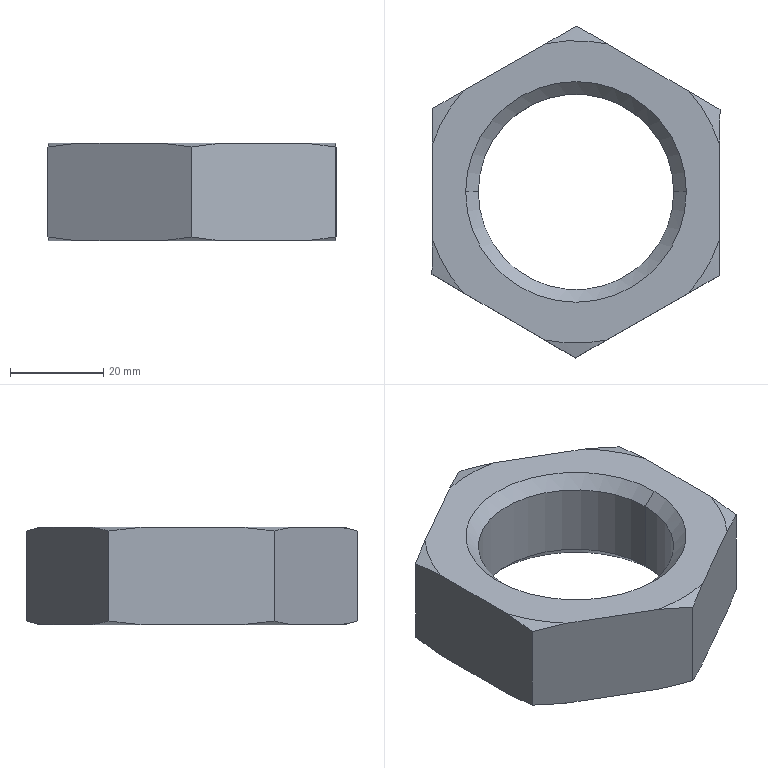Part | SolidWorks | features Cut 2, Chamfer 1, Extrusion 1 | 1 solid | 26 faces | box 61.887 x 71.299 x 21 mm | volume 39180 mm3 | cone 16 | plane 8 | cylinder 2 | commonest cylinder face diameters 42 x2
STEP:
#1=CARTESIAN_POINT('',(-21.,0.,18.3));
#2=VERTEX_POINT('',#1);
#3=CARTESIAN_POINT('',(21.,0.,18.3));
#4=VERTEX_POINT('',#3);
#5=CARTESIAN_POINT('',(0.,0.,18.3));
#6=DIRECTION('',(0.,0.,1.));
#7=DIRECTION('',(-1.,0.,0.));
#8=AXIS2_PLACEMENT_3D('',#5,#6,#7);
#9=CIRCLE('',#8,21.);
#10=EDGE_CURVE('',#2,#4,#9,.T.);
#11=ORIENTED_EDGE('',*,*,#10,.F.);
#12=CARTESIAN_POINT('',(-23.7,0.,21.));
#13=VERTEX_POINT('',#12);
#14=CARTESIAN_POINT('',(-21.,0.,18.3));
#15=DIRECTION('',(-0.7071,0.,0.7071));
#16=VECTOR('',#15,1000.);
#17=LINE('',#14,#16);
#18=EDGE_CURVE('',#2,#13,#17,.T.);
#19=ORIENTED_EDGE('',*,*,#18,.T.);
#20=CARTESIAN_POINT('',(23.7,0.,21.));
#21=VERTEX_POINT('',#20);
#22=CARTESIAN_POINT('',(0.,0.,21.));
#23=DIRECTION('',(0.,0.,-1.));
#24=DIRECTION('',(-1.,0.,0.));
#25=AXIS2_PLACEMENT_3D('',#22,#23,#24);
#26=CIRCLE('',#25,23.7);
#27=EDGE_CURVE('',#21,#13,#26,.T.);
#28=ORIENTED_EDGE('',*,*,#27,.F.);
#29=CARTESIAN_POINT('',(21.,0.,18.3));
#30=DIRECTION('',(0.7071,0.,0.7071));
#31=VECTOR('',#30,1000.);
#32=LINE('',#29,#31);
#33=EDGE_CURVE('',#4,#21,#32,.T.);
#34=ORIENTED_EDGE('',*,*,#33,.F.);
#35=EDGE_LOOP('',(#11,#19,#28,#34));
#36=FACE_OUTER_BOUND('',#35,.T.);
#37=CARTESIAN_POINT('',(0.,0.,18.3));
#38=DIRECTION('',(0.,0.,1.));
#39=DIRECTION('',(1.,0.,0.));
#40=AXIS2_PLACEMENT_3D('',#37,#38,#39);
#41=CONICAL_SURFACE('',#40,21.,0.7854);
#42=ADVANCED_FACE('',(#36),#41,.F.);
#43=CARTESIAN_POINT('',(21.,0.,2.7));
#44=VERTEX_POINT('',#43);
#45=CARTESIAN_POINT('',(-21.,0.,2.7));
#46=VERTEX_POINT('',#45);
#47=CARTESIAN_POINT('',(0.,0.,2.7));
#48=DIRECTION('',(0.,0.,-1.));
#49=DIRECTION('',(-1.,0.,0.));
#50=AXIS2_PLACEMENT_3D('',#47,#48,#49);
#51=CIRCLE('',#50,21.);
#52=EDGE_CURVE('',#44,#46,#51,.T.);
#53=ORIENTED_EDGE('',*,*,#52,.F.);
#54=CARTESIAN_POINT('',(23.7,0.,0.));
#55=VERTEX_POINT('',#54);
#56=CARTESIAN_POINT('',(23.7,0.,0.));
#57=DIRECTION('',(0.7071,0.,-0.7071));
#58=VECTOR('',#57,1000.);
#59=LINE('',#56,#58);
#60=EDGE_CURVE('',#44,#55,#59,.T.);
#61=ORIENTED_EDGE('',*,*,#60,.T.);
#62=CARTESIAN_POINT('',(-23.7,0.,0.));
#63=VERTEX_POINT('',#62);
#64=CARTESIAN_POINT('',(0.,0.,0.));
#65=DIRECTION('',(0.,0.,1.));
#66=DIRECTION('',(-1.,0.,0.));
#67=AXIS2_PLACEMENT_3D('',#64,#65,#66);
#68=CIRCLE('',#67,23.7);
#69=EDGE_CURVE('',#63,#55,#68,.T.);
#70=ORIENTED_EDGE('',*,*,#69,.F.);
#71=CARTESIAN_POINT('',(-23.7,0.,0.));
#72=DIRECTION('',(-0.7071,0.,-0.7071));
#73=VECTOR('',#72,1000.);
#74=LINE('',#71,#73);
#75=EDGE_CURVE('',#46,#63,#74,.T.);
#76=ORIENTED_EDGE('',*,*,#75,.F.);
#77=EDGE_LOOP('',(#53,#61,#70,#76));
#78=FACE_OUTER_BOUND('',#77,.T.);
#79=CARTESIAN_POINT('',(0.,0.,0.));
#80=DIRECTION('',(0.,0.,-1.));
#81=DIRECTION('',(-1.,0.,0.));
#82=AXIS2_PLACEMENT_3D('',#79,#80,#81);
#83=CONICAL_SURFACE('',#82,23.7,0.7854);
#84=ADVANCED_FACE('',(#78),#83,.F.);
#85=ORIENTED_EDGE('',*,*,#10,.T.);
#86=CARTESIAN_POINT('',(21.,0.,21.));
#87=DIRECTION('',(0.,0.,-1.));
#88=VECTOR('',#87,1000.);
#89=LINE('',#86,#88);
#90=EDGE_CURVE('',#4,#44,#89,.T.);
#91=ORIENTED_EDGE('',*,*,#90,.T.);
#92=ORIENTED_EDGE('',*,*,#52,.T.);
#93=CARTESIAN_POINT('',(-21.,0.,21.));
#94=DIRECTION('',(0.,0.,-1.));
#95=VECTOR('',#94,1000.);
#96=LINE('',#93,#95);
#97=EDGE_CURVE('',#2,#46,#96,.T.);
#98=ORIENTED_EDGE('',*,*,#97,.F.);
#99=EDGE_LOOP('',(#85,#91,#92,#98));
#100=FACE_OUTER_BOUND('',#99,.T.);
#101=CARTESIAN_POINT('',(0.,0.,21.));
#102=DIRECTION('',(0.,0.,-1.));
#103=DIRECTION('',(-1.,0.,0.));
#104=AXIS2_PLACEMENT_3D('',#101,#102,#103);
#105=CYLINDRICAL_SURFACE('',#104,21.);
#106=ADVANCED_FACE('',(#100),#105,.F.);
#107=CARTESIAN_POINT('',(30.944,17.703,20.156));
#108=VERTEX_POINT('',#107);
#109=CARTESIAN_POINT('',(24.314,21.566,21.));
#110=VERTEX_POINT('',#109);
#111=CARTESIAN_POINT('',(30.944,17.703,20.156));
#112=CARTESIAN_POINT('',(28.739,18.988,20.498));
#113=CARTESIAN_POINT('',(26.53,20.275,20.785));
#114=CARTESIAN_POINT('',(24.314,21.566,21.));
#115=B_SPLINE_CURVE_WITH_KNOTS('',3,(#111,#112,#113,#114),.UNSPECIFIED.,.F.,.F.,(4,4),(0.02915,0.03687),.UNSPECIFIED.);
#116=EDGE_CURVE('',#108,#110,#115,.T.);
#117=ORIENTED_EDGE('',*,*,#116,.F.);
#118=CARTESIAN_POINT('',(30.944,17.703,0.844));
#119=VERTEX_POINT('',#118);
#120=CARTESIAN_POINT('',(30.944,17.703,21.));
#121=DIRECTION('',(0.,0.,-1.));
#122=VECTOR('',#121,1000.);
#123=LINE('',#120,#122);
#124=EDGE_CURVE('',#108,#119,#123,.T.);
#125=ORIENTED_EDGE('',*,*,#124,.T.);
#126=CARTESIAN_POINT('',(24.314,21.566,0.));
#127=VERTEX_POINT('',#126);
#128=CARTESIAN_POINT('',(24.314,21.566,0.));
#129=CARTESIAN_POINT('',(26.533,20.273,0.215));
#130=CARTESIAN_POINT('',(28.743,18.986,0.5027));
#131=CARTESIAN_POINT('',(30.944,17.703,0.844));
#132=B_SPLINE_CURVE_WITH_KNOTS('',3,(#128,#129,#130,#131),.UNSPECIFIED.,.F.,.F.,(4,4),(0.05705,0.06464),.UNSPECIFIED.);
#133=EDGE_CURVE('',#127,#119,#132,.T.);
#134=ORIENTED_EDGE('',*,*,#133,.F.);
#135=CARTESIAN_POINT('',(6.77,31.787,0.));
#136=VERTEX_POINT('',#135);
#137=CARTESIAN_POINT('',(30.944,17.703,0.));
#138=DIRECTION('',(-0.8641,0.5034,0.));
#139=VECTOR('',#138,1000.);
#140=LINE('',#137,#139);
#141=EDGE_CURVE('',#127,#136,#140,.T.);
#142=ORIENTED_EDGE('',*,*,#141,.T.);
#143=CARTESIAN_POINT('',(0.1402,35.65,0.844));
#144=VERTEX_POINT('',#143);
#145=CARTESIAN_POINT('',(0.1402,35.65,0.844));
#146=CARTESIAN_POINT('',(2.345,34.365,0.5023));
#147=CARTESIAN_POINT('',(4.554,33.078,0.2147));
#148=CARTESIAN_POINT('',(6.77,31.787,0.));
#149=B_SPLINE_CURVE_WITH_KNOTS('',3,(#145,#146,#147,#148),.UNSPECIFIED.,.F.,.F.,(4,4),(0.02915,0.03687),.UNSPECIFIED.);
#150=EDGE_CURVE('',#144,#136,#149,.T.);
#151=ORIENTED_EDGE('',*,*,#150,.F.);
#152=CARTESIAN_POINT('',(0.1402,35.65,20.156));
#153=VERTEX_POINT('',#152);
#154=CARTESIAN_POINT('',(0.1402,35.65,21.));
#155=DIRECTION('',(0.,0.,-1.));
#156=VECTOR('',#155,1000.);
#157=LINE('',#154,#156);
#158=EDGE_CURVE('',#153,#144,#157,.T.);
#159=ORIENTED_EDGE('',*,*,#158,.F.);
#160=CARTESIAN_POINT('',(6.77,31.787,21.));
#161=VERTEX_POINT('',#160);
#162=CARTESIAN_POINT('',(6.77,31.787,21.));
#163=CARTESIAN_POINT('',(4.551,33.08,20.785));
#164=CARTESIAN_POINT('',(2.341,34.367,20.497));
#165=CARTESIAN_POINT('',(0.1402,35.65,20.156));
#166=B_SPLINE_CURVE_WITH_KNOTS('',3,(#162,#163,#164,#165),.UNSPECIFIED.,.F.,.F.,(4,4),(0.05705,0.06464),.UNSPECIFIED.);
#167=EDGE_CURVE('',#161,#153,#166,.T.);
#168=ORIENTED_EDGE('',*,*,#167,.F.);
#169=CARTESIAN_POINT('',(30.944,17.703,21.));
#170=DIRECTION('',(-0.8641,0.5034,0.));
#171=VECTOR('',#170,1000.);
#172=LINE('',#169,#171);
#173=EDGE_CURVE('',#110,#161,#172,.T.);
#174=ORIENTED_EDGE('',*,*,#173,.F.);
#175=EDGE_LOOP('',(#117,#125,#134,#142,#151,#159,#168,#174));
#176=FACE_OUTER_BOUND('',#175,.T.);
#177=CARTESIAN_POINT('',(30.944,17.703,21.));
#178=DIRECTION('',(-0.5034,-0.8641,0.));
#179=DIRECTION('',(0.8641,-0.5034,0.));
#180=AXIS2_PLACEMENT_3D('',#177,#178,#179);
#181=PLANE('',#180);
#182=ADVANCED_FACE('',(#176),#181,.F.);
#183=CARTESIAN_POINT('',(-6.52,31.839,21.));
#184=VERTEX_POINT('',#183);
#185=CARTESIAN_POINT('',(0.1402,35.65,20.156));
#186=CARTESIAN_POINT('',(-2.074,34.383,20.498));
#187=CARTESIAN_POINT('',(-4.294,33.113,20.785));
#188=CARTESIAN_POINT('',(-6.52,31.839,21.));
#189=B_SPLINE_CURVE_WITH_KNOTS('',3,(#185,#186,#187,#188),.UNSPECIFIED.,.F.,.F.,(4,4),(0.02902,0.03674),.UNSPECIFIED.);
#190=EDGE_CURVE('',#153,#184,#189,.T.);
#191=ORIENTED_EDGE('',*,*,#190,.F.);
#192=ORIENTED_EDGE('',*,*,#158,.T.);
#193=CARTESIAN_POINT('',(-6.52,31.839,0.));
#194=VERTEX_POINT('',#193);
#195=CARTESIAN_POINT('',(-6.52,31.839,0.));
#196=CARTESIAN_POINT('',(-4.291,33.115,0.215));
#197=CARTESIAN_POINT('',(-2.071,34.385,0.5027));
#198=CARTESIAN_POINT('',(0.1402,35.65,0.844));
#199=B_SPLINE_CURVE_WITH_KNOTS('',3,(#195,#196,#197,#198),.UNSPECIFIED.,.F.,.F.,(4,4),(0.05692,0.06451),.UNSPECIFIED.);
#200=EDGE_CURVE('',#194,#144,#199,.T.);
#201=ORIENTED_EDGE('',*,*,#200,.F.);
#202=CARTESIAN_POINT('',(-24.143,21.757,0.));
#203=VERTEX_POINT('',#202);
#204=CARTESIAN_POINT('',(0.1402,35.65,0.));
#205=DIRECTION('',(-0.868,-0.4966,0.));
#206=VECTOR('',#205,1000.);
#207=LINE('',#204,#206);
#208=EDGE_CURVE('',#194,#203,#207,.T.);
#209=ORIENTED_EDGE('',*,*,#208,.T.);
#210=CARTESIAN_POINT('',(-30.803,17.946,0.844));
#211=VERTEX_POINT('',#210);
#212=CARTESIAN_POINT('',(-30.803,17.946,0.844));
#213=CARTESIAN_POINT('',(-28.589,19.213,0.5023));
#214=CARTESIAN_POINT('',(-26.37,20.483,0.2147));
#215=CARTESIAN_POINT('',(-24.143,21.757,0.));
#216=B_SPLINE_CURVE_WITH_KNOTS('',3,(#212,#213,#214,#215),.UNSPECIFIED.,.F.,.F.,(4,4),(0.02902,0.03674),.UNSPECIFIED.);
#217=EDGE_CURVE('',#211,#203,#216,.T.);
#218=ORIENTED_EDGE('',*,*,#217,.F.);
#219=CARTESIAN_POINT('',(-30.803,17.946,20.156));
#220=VERTEX_POINT('',#219);
#221=CARTESIAN_POINT('',(-30.803,17.946,21.));
#222=DIRECTION('',(0.,0.,-1.));
#223=VECTOR('',#222,1000.);
#224=LINE('',#221,#223);
#225=EDGE_CURVE('',#220,#211,#224,.T.);
#226=ORIENTED_EDGE('',*,*,#225,.F.);
#227=CARTESIAN_POINT('',(-24.143,21.757,21.));
#228=VERTEX_POINT('',#227);
#229=CARTESIAN_POINT('',(-24.143,21.757,21.));
#230=CARTESIAN_POINT('',(-26.372,20.481,20.785));
#231=CARTESIAN_POINT('',(-28.592,19.211,20.497));
#232=CARTESIAN_POINT('',(-30.803,17.946,20.156));
#233=B_SPLINE_CURVE_WITH_KNOTS('',3,(#229,#230,#231,#232),.UNSPECIFIED.,.F.,.F.,(4,4),(0.05692,0.06451),.UNSPECIFIED.);
#234=EDGE_CURVE('',#228,#220,#233,.T.);
#235=ORIENTED_EDGE('',*,*,#234,.F.);
#236=CARTESIAN_POINT('',(0.1402,35.65,21.));
#237=DIRECTION('',(-0.868,-0.4966,0.));
#238=VECTOR('',#237,1000.);
#239=LINE('',#236,#238);
#240=EDGE_CURVE('',#184,#228,#239,.T.);
#241=ORIENTED_EDGE('',*,*,#240,.F.);
#242=EDGE_LOOP('',(#191,#192,#201,#209,#218,#226,#235,#241));
#243=FACE_OUTER_BOUND('',#242,.T.);
#244=CARTESIAN_POINT('',(0.1402,35.65,21.));
#245=DIRECTION('',(0.4966,-0.868,0.));
#246=DIRECTION('',(0.868,0.4966,0.));
#247=AXIS2_PLACEMENT_3D('',#244,#245,#246);
#248=PLANE('',#247);
#249=ADVANCED_FACE('',(#243),#248,.F.);
#250=CARTESIAN_POINT('',(-30.834,10.273,21.));
#251=VERTEX_POINT('',#250);
#252=CARTESIAN_POINT('',(-30.803,17.946,20.156));
#253=CARTESIAN_POINT('',(-30.813,15.395,20.498));
#254=CARTESIAN_POINT('',(-30.824,12.837,20.785));
#255=CARTESIAN_POINT('',(-30.834,10.273,21.));
#256=B_SPLINE_CURVE_WITH_KNOTS('',3,(#252,#253,#254,#255),.UNSPECIFIED.,.F.,.F.,(4,4),(0.02515,0.03287),.UNSPECIFIED.);
#257=EDGE_CURVE('',#220,#251,#256,.T.);
#258=ORIENTED_EDGE('',*,*,#257,.F.);
#259=ORIENTED_EDGE('',*,*,#225,.T.);
#260=CARTESIAN_POINT('',(-30.834,10.273,0.));
#261=VERTEX_POINT('',#260);
#262=CARTESIAN_POINT('',(-30.834,10.273,0.));
#263=CARTESIAN_POINT('',(-30.829,11.556,0.1073));
#264=CARTESIAN_POINT('',(-30.824,12.838,0.2331));
#265=CARTESIAN_POINT('',(-30.813,15.396,0.5161));
#266=CARTESIAN_POINT('',(-30.808,16.672,0.6734));
#267=CARTESIAN_POINT('',(-30.803,17.946,0.844));
#268=B_SPLINE_CURVE_WITH_KNOTS('',3,(#262,#263,#264,#265,#266,#267),.UNSPECIFIED.,.F.,.F.,(4,2,4),(0.05308,0.05687,0.06067),.UNSPECIFIED.);
#269=EDGE_CURVE('',#261,#211,#268,.T.);
#270=ORIENTED_EDGE('',*,*,#269,.F.);
#271=CARTESIAN_POINT('',(-30.914,-10.03,0.));
#272=VERTEX_POINT('',#271);
#273=CARTESIAN_POINT('',(-30.803,17.946,0.));
#274=DIRECTION('',(-0.003934,-1.,0.));
#275=VECTOR('',#274,1000.);
#276=LINE('',#273,#275);
#277=EDGE_CURVE('',#261,#272,#276,.T.);
#278=ORIENTED_EDGE('',*,*,#277,.T.);
#279=CARTESIAN_POINT('',(-30.944,-17.703,0.844));
#280=VERTEX_POINT('',#279);
#281=CARTESIAN_POINT('',(-30.944,-17.703,0.844));
#282=CARTESIAN_POINT('',(-30.934,-15.152,0.5022));
#283=CARTESIAN_POINT('',(-30.924,-12.595,0.2146));
#284=CARTESIAN_POINT('',(-30.914,-10.03,0.));
#285=B_SPLINE_CURVE_WITH_KNOTS('',3,(#281,#282,#283,#284),.UNSPECIFIED.,.F.,.F.,(4,4),(0.02515,0.03287),.UNSPECIFIED.);
#286=EDGE_CURVE('',#280,#272,#285,.T.);
#287=ORIENTED_EDGE('',*,*,#286,.F.);
#288=CARTESIAN_POINT('',(-30.944,-17.703,20.156));
#289=VERTEX_POINT('',#288);
#290=CARTESIAN_POINT('',(-30.944,-17.703,21.));
#291=DIRECTION('',(0.,0.,-1.));
#292=VECTOR('',#291,1000.);
#293=LINE('',#290,#292);
#294=EDGE_CURVE('',#289,#280,#293,.T.);
#295=ORIENTED_EDGE('',*,*,#294,.F.);
#296=CARTESIAN_POINT('',(-30.914,-10.03,21.));
#297=VERTEX_POINT('',#296);
#298=CARTESIAN_POINT('',(-30.914,-10.03,21.));
#299=CARTESIAN_POINT('',(-30.919,-11.313,20.893));
#300=CARTESIAN_POINT('',(-30.924,-12.596,20.767));
#301=CARTESIAN_POINT('',(-30.934,-15.153,20.484));
#302=CARTESIAN_POINT('',(-30.939,-16.429,20.327));
#303=CARTESIAN_POINT('',(-30.944,-17.703,20.156));
#304=B_SPLINE_CURVE_WITH_KNOTS('',3,(#298,#299,#300,#301,#302,#303),.UNSPECIFIED.,.F.,.F.,(4,2,4),(0.05308,0.05687,0.06067),.UNSPECIFIED.);
#305=EDGE_CURVE('',#297,#289,#304,.T.);
#306=ORIENTED_EDGE('',*,*,#305,.F.);
#307=CARTESIAN_POINT('',(-30.803,17.946,21.));
#308=DIRECTION('',(-0.003934,-1.,0.));
#309=VECTOR('',#308,1000.);
#310=LINE('',#307,#309);
#311=EDGE_CURVE('',#251,#297,#310,.T.);
#312=ORIENTED_EDGE('',*,*,#311,.F.);
#313=EDGE_LOOP('',(#258,#259,#270,#278,#287,#295,#306,#312));
#314=FACE_OUTER_BOUND('',#313,.T.);
#315=CARTESIAN_POINT('',(-30.803,17.946,21.));
#316=DIRECTION('',(1.,-0.003934,0.));
#317=DIRECTION('',(0.003934,1.,0.));
#318=AXIS2_PLACEMENT_3D('',#315,#316,#317);
#319=PLANE('',#318);
#320=ADVANCED_FACE('',(#314),#319,.F.);
#321=CARTESIAN_POINT('',(-24.314,-21.566,21.));
#322=VERTEX_POINT('',#321);
#323=CARTESIAN_POINT('',(-30.944,-17.703,20.156));
#324=CARTESIAN_POINT('',(-28.739,-18.988,20.498));
#325=CARTESIAN_POINT('',(-26.53,-20.275,20.785));
#326=CARTESIAN_POINT('',(-24.314,-21.566,21.));
#327=B_SPLINE_CURVE_WITH_KNOTS('',3,(#323,#324,#325,#326),.UNSPECIFIED.,.F.,.F.,(4,4),(0.02915,0.03687),.UNSPECIFIED.);
#328=EDGE_CURVE('',#289,#322,#327,.T.);
#329=ORIENTED_EDGE('',*,*,#328,.F.);
#330=ORIENTED_EDGE('',*,*,#294,.T.);
#331=CARTESIAN_POINT('',(-24.314,-21.566,0.));
#332=VERTEX_POINT('',#331);
#333=CARTESIAN_POINT('',(-24.314,-21.566,0.));
#334=CARTESIAN_POINT('',(-26.533,-20.273,0.215));
#335=CARTESIAN_POINT('',(-28.743,-18.986,0.5027));
#336=CARTESIAN_POINT('',(-30.944,-17.703,0.844));
#337=B_SPLINE_CURVE_WITH_KNOTS('',3,(#333,#334,#335,#336),.UNSPECIFIED.,.F.,.F.,(4,4),(0.05705,0.06464),.UNSPECIFIED.);
#338=EDGE_CURVE('',#332,#280,#337,.T.);
#339=ORIENTED_EDGE('',*,*,#338,.F.);
#340=CARTESIAN_POINT('',(-6.77,-31.787,0.));
#341=VERTEX_POINT('',#340);
#342=CARTESIAN_POINT('',(-30.944,-17.703,0.));
#343=DIRECTION('',(0.8641,-0.5034,0.));
#344=VECTOR('',#343,1000.);
#345=LINE('',#342,#344);
#346=EDGE_CURVE('',#332,#341,#345,.T.);
#347=ORIENTED_EDGE('',*,*,#346,.T.);
#348=CARTESIAN_POINT('',(-0.1402,-35.65,0.844));
#349=VERTEX_POINT('',#348);
#350=CARTESIAN_POINT('',(-0.1402,-35.65,0.844));
#351=CARTESIAN_POINT('',(-2.345,-34.365,0.5023));
#352=CARTESIAN_POINT('',(-4.554,-33.078,0.2147));
#353=CARTESIAN_POINT('',(-6.77,-31.787,0.));
#354=B_SPLINE_CURVE_WITH_KNOTS('',3,(#350,#351,#352,#353),.UNSPECIFIED.,.F.,.F.,(4,4),(0.02915,0.03687),.UNSPECIFIED.);
#355=EDGE_CURVE('',#349,#341,#354,.T.);
#356=ORIENTED_EDGE('',*,*,#355,.F.);
#357=CARTESIAN_POINT('',(-0.1402,-35.65,20.156));
#358=VERTEX_POINT('',#357);
#359=CARTESIAN_POINT('',(-0.1402,-35.65,21.));
#360=DIRECTION('',(0.,0.,-1.));
#361=VECTOR('',#360,1000.);
#362=LINE('',#359,#361);
#363=EDGE_CURVE('',#358,#349,#362,.T.);
#364=ORIENTED_EDGE('',*,*,#363,.F.);
#365=CARTESIAN_POINT('',(-6.77,-31.787,21.));
#366=VERTEX_POINT('',#365);
#367=CARTESIAN_POINT('',(-6.77,-31.787,21.));
#368=CARTESIAN_POINT('',(-4.551,-33.08,20.785));
#369=CARTESIAN_POINT('',(-2.341,-34.367,20.497));
#370=CARTESIAN_POINT('',(-0.1402,-35.65,20.156));
#371=B_SPLINE_CURVE_WITH_KNOTS('',3,(#367,#368,#369,#370),.UNSPECIFIED.,.F.,.F.,(4,4),(0.05705,0.06464),.UNSPECIFIED.);
#372=EDGE_CURVE('',#366,#358,#371,.T.);
#373=ORIENTED_EDGE('',*,*,#372,.F.);
#374=CARTESIAN_POINT('',(-30.944,-17.703,21.));
#375=DIRECTION('',(0.8641,-0.5034,0.));
#376=VECTOR('',#375,1000.);
#377=LINE('',#374,#376);
#378=EDGE_CURVE('',#322,#366,#377,.T.);
#379=ORIENTED_EDGE('',*,*,#378,.F.);
#380=EDGE_LOOP('',(#329,#330,#339,#347,#356,#364,#373,#379));
#381=FACE_OUTER_BOUND('',#380,.T.);
#382=CARTESIAN_POINT('',(-30.944,-17.703,21.));
#383=DIRECTION('',(0.5034,0.8641,0.));
#384=DIRECTION('',(-0.8641,0.5034,0.));
#385=AXIS2_PLACEMENT_3D('',#382,#383,#384);
#386=PLANE('',#385);
#387=ADVANCED_FACE('',(#381),#386,.F.);
#388=CARTESIAN_POINT('',(6.52,-31.839,21.));
#389=VERTEX_POINT('',#388);
#390=CARTESIAN_POINT('',(-0.1402,-35.65,20.156));
#391=CARTESIAN_POINT('',(2.074,-34.383,20.498));
#392=CARTESIAN_POINT('',(4.294,-33.113,20.785));
#393=CARTESIAN_POINT('',(6.52,-31.839,21.));
#394=B_SPLINE_CURVE_WITH_KNOTS('',3,(#390,#391,#392,#393),.UNSPECIFIED.,.F.,.F.,(4,4),(0.02902,0.03674),.UNSPECIFIED.);
#395=EDGE_CURVE('',#358,#389,#394,.T.);
#396=ORIENTED_EDGE('',*,*,#395,.F.);
#397=ORIENTED_EDGE('',*,*,#363,.T.);
#398=CARTESIAN_POINT('',(6.52,-31.839,0.));
#399=VERTEX_POINT('',#398);
#400=CARTESIAN_POINT('',(6.52,-31.839,0.));
#401=CARTESIAN_POINT('',(4.291,-33.115,0.215));
#402=CARTESIAN_POINT('',(2.071,-34.385,0.5027));
#403=CARTESIAN_POINT('',(-0.1402,-35.65,0.844));
#404=B_SPLINE_CURVE_WITH_KNOTS('',3,(#400,#401,#402,#403),.UNSPECIFIED.,.F.,.F.,(4,4),(0.05692,0.06451),.UNSPECIFIED.);
#405=EDGE_CURVE('',#399,#349,#404,.T.);
#406=ORIENTED_EDGE('',*,*,#405,.F.);
#407=CARTESIAN_POINT('',(24.143,-21.757,0.));
#408=VERTEX_POINT('',#407);
#409=CARTESIAN_POINT('',(-0.1402,-35.65,0.));
#410=DIRECTION('',(0.868,0.4966,0.));
#411=VECTOR('',#410,1000.);
#412=LINE('',#409,#411);
#413=EDGE_CURVE('',#399,#408,#412,.T.);
#414=ORIENTED_EDGE('',*,*,#413,.T.);
#415=CARTESIAN_POINT('',(30.803,-17.946,0.844));
#416=VERTEX_POINT('',#415);
#417=CARTESIAN_POINT('',(30.803,-17.946,0.844));
#418=CARTESIAN_POINT('',(28.589,-19.213,0.5023));
#419=CARTESIAN_POINT('',(26.37,-20.483,0.2147));
#420=CARTESIAN_POINT('',(24.143,-21.757,0.));
#421=B_SPLINE_CURVE_WITH_KNOTS('',3,(#417,#418,#419,#420),.UNSPECIFIED.,.F.,.F.,(4,4),(0.02902,0.03674),.UNSPECIFIED.);
#422=EDGE_CURVE('',#416,#408,#421,.T.);
#423=ORIENTED_EDGE('',*,*,#422,.F.);
#424=CARTESIAN_POINT('',(30.803,-17.946,20.156));
#425=VERTEX_POINT('',#424);
#426=CARTESIAN_POINT('',(30.803,-17.946,21.));
#427=DIRECTION('',(0.,0.,-1.));
#428=VECTOR('',#427,1000.);
#429=LINE('',#426,#428);
#430=EDGE_CURVE('',#425,#416,#429,.T.);
#431=ORIENTED_EDGE('',*,*,#430,.F.);
#432=CARTESIAN_POINT('',(24.143,-21.757,21.));
#433=VERTEX_POINT('',#432);
#434=CARTESIAN_POINT('',(24.143,-21.757,21.));
#435=CARTESIAN_POINT('',(26.372,-20.481,20.785));
#436=CARTESIAN_POINT('',(28.592,-19.211,20.497));
#437=CARTESIAN_POINT('',(30.803,-17.946,20.156));
#438=B_SPLINE_CURVE_WITH_KNOTS('',3,(#434,#435,#436,#437),.UNSPECIFIED.,.F.,.F.,(4,4),(0.05692,0.06451),.UNSPECIFIED.);
#439=EDGE_CURVE('',#433,#425,#438,.T.);
#440=ORIENTED_EDGE('',*,*,#439,.F.);
#441=CARTESIAN_POINT('',(-0.1402,-35.65,21.));
#442=DIRECTION('',(0.868,0.4966,0.));
#443=VECTOR('',#442,1000.);
#444=LINE('',#441,#443);
#445=EDGE_CURVE('',#389,#433,#444,.T.);
#446=ORIENTED_EDGE('',*,*,#445,.F.);
#447=EDGE_LOOP('',(#396,#397,#406,#414,#423,#431,#440,#446));
#448=FACE_OUTER_BOUND('',#447,.T.);
#449=CARTESIAN_POINT('',(-0.1402,-35.65,21.));
#450=DIRECTION('',(-0.4966,0.868,0.));
#451=DIRECTION('',(-0.868,-0.4966,0.));
#452=AXIS2_PLACEMENT_3D('',#449,#450,#451);
#453=PLANE('',#452);
#454=ADVANCED_FACE('',(#448),#453,.F.);
#455=CARTESIAN_POINT('',(30.834,-10.273,21.));
#456=VERTEX_POINT('',#455);
#457=CARTESIAN_POINT('',(30.803,-17.946,20.156));
#458=CARTESIAN_POINT('',(30.813,-15.395,20.498));
#459=CARTESIAN_POINT('',(30.824,-12.837,20.785));
#460=CARTESIAN_POINT('',(30.834,-10.273,21.));
#461=B_SPLINE_CURVE_WITH_KNOTS('',3,(#457,#458,#459,#460),.UNSPECIFIED.,.F.,.F.,(4,4),(0.02515,0.03287),.UNSPECIFIED.);
#462=EDGE_CURVE('',#425,#456,#461,.T.);
#463=ORIENTED_EDGE('',*,*,#462,.F.);
#464=ORIENTED_EDGE('',*,*,#430,.T.);
#465=CARTESIAN_POINT('',(30.834,-10.273,0.));
#466=VERTEX_POINT('',#465);
#467=CARTESIAN_POINT('',(30.834,-10.273,0.));
#468=CARTESIAN_POINT('',(30.829,-11.556,0.1073));
#469=CARTESIAN_POINT('',(30.824,-12.838,0.2331));
#470=CARTESIAN_POINT('',(30.813,-15.396,0.5161));
#471=CARTESIAN_POINT('',(30.808,-16.672,0.6734));
#472=CARTESIAN_POINT('',(30.803,-17.946,0.844));
#473=B_SPLINE_CURVE_WITH_KNOTS('',3,(#467,#468,#469,#470,#471,#472),.UNSPECIFIED.,.F.,.F.,(4,2,4),(0.05308,0.05687,0.06067),.UNSPECIFIED.);
#474=EDGE_CURVE('',#466,#416,#473,.T.);
#475=ORIENTED_EDGE('',*,*,#474,.F.);
#476=CARTESIAN_POINT('',(30.914,10.03,0.));
#477=VERTEX_POINT('',#476);
#478=CARTESIAN_POINT('',(30.803,-17.946,0.));
#479=DIRECTION('',(0.003934,1.,0.));
#480=VECTOR('',#479,1000.);
#481=LINE('',#478,#480);
#482=EDGE_CURVE('',#466,#477,#481,.T.);
#483=ORIENTED_EDGE('',*,*,#482,.T.);
#484=CARTESIAN_POINT('',(30.944,17.703,0.844));
#485=CARTESIAN_POINT('',(30.934,15.152,0.5022));
#486=CARTESIAN_POINT('',(30.924,12.595,0.2146));
#487=CARTESIAN_POINT('',(30.914,10.03,0.));
#488=B_SPLINE_CURVE_WITH_KNOTS('',3,(#484,#485,#486,#487),.UNSPECIFIED.,.F.,.F.,(4,4),(0.02515,0.03287),.UNSPECIFIED.);
#489=EDGE_CURVE('',#119,#477,#488,.T.);
#490=ORIENTED_EDGE('',*,*,#489,.F.);
#491=ORIENTED_EDGE('',*,*,#124,.F.);
#492=CARTESIAN_POINT('',(30.914,10.03,21.));
#493=VERTEX_POINT('',#492);
#494=CARTESIAN_POINT('',(30.914,10.03,21.));
#495=CARTESIAN_POINT('',(30.919,11.313,20.893));
#496=CARTESIAN_POINT('',(30.924,12.596,20.767));
#497=CARTESIAN_POINT('',(30.934,15.153,20.484));
#498=CARTESIAN_POINT('',(30.939,16.429,20.327));
#499=CARTESIAN_POINT('',(30.944,17.703,20.156));
#500=B_SPLINE_CURVE_WITH_KNOTS('',3,(#494,#495,#496,#497,#498,#499),.UNSPECIFIED.,.F.,.F.,(4,2,4),(0.05308,0.05687,0.06067),.UNSPECIFIED.);
#501=EDGE_CURVE('',#493,#108,#500,.T.);
#502=ORIENTED_EDGE('',*,*,#501,.F.);
#503=CARTESIAN_POINT('',(30.803,-17.946,21.));
#504=DIRECTION('',(0.003934,1.,0.));
#505=VECTOR('',#504,1000.);
#506=LINE('',#503,#505);
#507=EDGE_CURVE('',#456,#493,#506,.T.);
#508=ORIENTED_EDGE('',*,*,#507,.F.);
#509=EDGE_LOOP('',(#463,#464,#475,#483,#490,#491,#502,#508));
#510=FACE_OUTER_BOUND('',#509,.T.);
#511=CARTESIAN_POINT('',(30.803,-17.946,21.));
#512=DIRECTION('',(-1.,0.003934,0.));
#513=DIRECTION('',(-0.003934,-1.,0.));
#514=AXIS2_PLACEMENT_3D('',#511,#512,#513);
#515=PLANE('',#514);
#516=ADVANCED_FACE('',(#510),#515,.F.);
#517=ORIENTED_EDGE('',*,*,#27,.T.);
#518=CARTESIAN_POINT('',(0.,0.,21.));
#519=DIRECTION('',(0.,0.,-1.));
#520=DIRECTION('',(-1.,0.,0.));
#521=AXIS2_PLACEMENT_3D('',#518,#519,#520);
#522=CIRCLE('',#521,23.7);
#523=EDGE_CURVE('',#13,#21,#522,.T.);
#524=ORIENTED_EDGE('',*,*,#523,.T.);
#525=EDGE_LOOP('',(#517,#524));
#526=FACE_BOUND('',#525,.T.);
#527=CARTESIAN_POINT('',(0.,0.,21.));
#528=DIRECTION('',(0.,0.,-1.));
#529=DIRECTION('',(-1.,0.,0.));
#530=AXIS2_PLACEMENT_3D('',#527,#528,#529);
#531=CIRCLE('',#530,32.5);
#532=EDGE_CURVE('',#251,#228,#531,.T.);
#533=ORIENTED_EDGE('',*,*,#532,.F.);
#534=ORIENTED_EDGE('',*,*,#311,.T.);
#535=CARTESIAN_POINT('',(0.,0.,21.));
#536=DIRECTION('',(0.,0.,-1.));
#537=DIRECTION('',(-1.,0.,0.));
#538=AXIS2_PLACEMENT_3D('',#535,#536,#537);
#539=CIRCLE('',#538,32.5);
#540=EDGE_CURVE('',#322,#297,#539,.T.);
#541=ORIENTED_EDGE('',*,*,#540,.F.);
#542=ORIENTED_EDGE('',*,*,#378,.T.);
#543=CARTESIAN_POINT('',(0.,0.,21.));
#544=DIRECTION('',(0.,0.,-1.));
#545=DIRECTION('',(-1.,0.,0.));
#546=AXIS2_PLACEMENT_3D('',#543,#544,#545);
#547=CIRCLE('',#546,32.5);
#548=EDGE_CURVE('',#389,#366,#547,.T.);
#549=ORIENTED_EDGE('',*,*,#548,.F.);
#550=ORIENTED_EDGE('',*,*,#445,.T.);
#551=CARTESIAN_POINT('',(0.,0.,21.));
#552=DIRECTION('',(0.,0.,-1.));
#553=DIRECTION('',(-1.,0.,0.));
#554=AXIS2_PLACEMENT_3D('',#551,#552,#553);
#555=CIRCLE('',#554,32.5);
#556=EDGE_CURVE('',#456,#433,#555,.T.);
#557=ORIENTED_EDGE('',*,*,#556,.F.);
#558=ORIENTED_EDGE('',*,*,#507,.T.);
#559=CARTESIAN_POINT('',(0.,0.,21.));
#560=DIRECTION('',(0.,0.,1.));
#561=DIRECTION('',(1.,0.,0.));
#562=AXIS2_PLACEMENT_3D('',#559,#560,#561);
#563=CIRCLE('',#562,32.5);
#564=EDGE_CURVE('',#493,#110,#563,.T.);
#565=ORIENTED_EDGE('',*,*,#564,.T.);
#566=ORIENTED_EDGE('',*,*,#173,.T.);
#567=CARTESIAN_POINT('',(0.,0.,21.));
#568=DIRECTION('',(0.,0.,-1.));
#569=DIRECTION('',(-1.,0.,0.));
#570=AXIS2_PLACEMENT_3D('',#567,#568,#569);
#571=CIRCLE('',#570,32.5);
#572=EDGE_CURVE('',#184,#161,#571,.T.);
#573=ORIENTED_EDGE('',*,*,#572,.F.);
#574=ORIENTED_EDGE('',*,*,#240,.T.);
#575=EDGE_LOOP('',(#533,#534,#541,#542,#549,#550,#557,#558,#565,#566,#573,#574));
#576=FACE_OUTER_BOUND('',#575,.T.);
#577=CARTESIAN_POINT('',(61.747,-0.2429,21.));
#578=DIRECTION('',(0.,0.,-1.));
#579=DIRECTION('',(-1.,0.,0.));
#580=AXIS2_PLACEMENT_3D('',#577,#578,#579);
#581=PLANE('',#580);
#582=ADVANCED_FACE('',(#526,#576),#581,.F.);
#583=ORIENTED_EDGE('',*,*,#69,.T.);
#584=CARTESIAN_POINT('',(0.,0.,0.));
#585=DIRECTION('',(0.,0.,1.));
#586=DIRECTION('',(-1.,0.,0.));
#587=AXIS2_PLACEMENT_3D('',#584,#585,#586);
#588=CIRCLE('',#587,23.7);
#589=EDGE_CURVE('',#55,#63,#588,.T.);
#590=ORIENTED_EDGE('',*,*,#589,.T.);
#591=EDGE_LOOP('',(#583,#590));
#592=FACE_BOUND('',#591,.T.);
#593=ORIENTED_EDGE('',*,*,#277,.F.);
#594=CARTESIAN_POINT('',(0.,0.,0.));
#595=DIRECTION('',(0.,0.,-1.));
#596=DIRECTION('',(-1.,0.,0.));
#597=AXIS2_PLACEMENT_3D('',#594,#595,#596);
#598=CIRCLE('',#597,32.5);
#599=EDGE_CURVE('',#261,#203,#598,.T.);
#600=ORIENTED_EDGE('',*,*,#599,.T.);
#601=ORIENTED_EDGE('',*,*,#208,.F.);
#602=CARTESIAN_POINT('',(0.,0.,0.));
#603=DIRECTION('',(0.,0.,-1.));
#604=DIRECTION('',(-1.,0.,0.));
#605=AXIS2_PLACEMENT_3D('',#602,#603,#604);
#606=CIRCLE('',#605,32.5);
#607=EDGE_CURVE('',#194,#136,#606,.T.);
#608=ORIENTED_EDGE('',*,*,#607,.T.);
#609=ORIENTED_EDGE('',*,*,#141,.F.);
#610=CARTESIAN_POINT('',(0.,0.,0.));
#611=DIRECTION('',(0.,0.,-1.));
#612=DIRECTION('',(-1.,0.,0.));
#613=AXIS2_PLACEMENT_3D('',#610,#611,#612);
#614=CIRCLE('',#613,32.5);
#615=EDGE_CURVE('',#127,#477,#614,.T.);
#616=ORIENTED_EDGE('',*,*,#615,.T.);
#617=ORIENTED_EDGE('',*,*,#482,.F.);
#618=CARTESIAN_POINT('',(0.,0.,0.));
#619=DIRECTION('',(0.,0.,-1.));
#620=DIRECTION('',(-1.,0.,0.));
#621=AXIS2_PLACEMENT_3D('',#618,#619,#620);
#622=CIRCLE('',#621,32.5);
#623=EDGE_CURVE('',#466,#408,#622,.T.);
#624=ORIENTED_EDGE('',*,*,#623,.T.);
#625=ORIENTED_EDGE('',*,*,#413,.F.);
#626=CARTESIAN_POINT('',(0.,0.,0.));
#627=DIRECTION('',(0.,0.,-1.));
#628=DIRECTION('',(-1.,0.,0.));
#629=AXIS2_PLACEMENT_3D('',#626,#627,#628);
#630=CIRCLE('',#629,32.5);
#631=EDGE_CURVE('',#399,#341,#630,.T.);
#632=ORIENTED_EDGE('',*,*,#631,.T.);
#633=ORIENTED_EDGE('',*,*,#346,.F.);
#634=CARTESIAN_POINT('',(0.,0.,0.));
#635=DIRECTION('',(0.,0.,-1.));
#636=DIRECTION('',(-1.,0.,0.));
#637=AXIS2_PLACEMENT_3D('',#634,#635,#636);
#638=CIRCLE('',#637,32.5);
#639=EDGE_CURVE('',#332,#272,#638,.T.);
#640=ORIENTED_EDGE('',*,*,#639,.T.);
#641=EDGE_LOOP('',(#593,#600,#601,#608,#609,#616,#617,#624,#625,#632,#633,#640));
#642=FACE_OUTER_BOUND('',#641,.T.);
#643=CARTESIAN_POINT('',(61.747,-0.2429,0.));
#644=DIRECTION('',(0.,0.,-1.));
#645=DIRECTION('',(-1.,0.,0.));
#646=AXIS2_PLACEMENT_3D('',#643,#644,#645);
#647=PLANE('',#646);
#648=ADVANCED_FACE('',(#592,#642),#647,.T.);
#649=ORIENTED_EDGE('',*,*,#90,.F.);
#650=CARTESIAN_POINT('',(0.,0.,18.3));
#651=DIRECTION('',(0.,0.,1.));
#652=DIRECTION('',(-1.,0.,0.));
#653=AXIS2_PLACEMENT_3D('',#650,#651,#652);
#654=CIRCLE('',#653,21.);
#655=EDGE_CURVE('',#4,#2,#654,.T.);
#656=ORIENTED_EDGE('',*,*,#655,.T.);
#657=ORIENTED_EDGE('',*,*,#97,.T.);
#658=CARTESIAN_POINT('',(0.,0.,2.7));
#659=DIRECTION('',(0.,0.,-1.));
#660=DIRECTION('',(-1.,0.,0.));
#661=AXIS2_PLACEMENT_3D('',#658,#659,#660);
#662=CIRCLE('',#661,21.);
#663=EDGE_CURVE('',#46,#44,#662,.T.);
#664=ORIENTED_EDGE('',*,*,#663,.T.);
#665=EDGE_LOOP('',(#649,#656,#657,#664));
#666=FACE_OUTER_BOUND('',#665,.T.);
#667=CARTESIAN_POINT('',(0.,0.,21.));
#668=DIRECTION('',(0.,0.,-1.));
#669=DIRECTION('',(-1.,0.,0.));
#670=AXIS2_PLACEMENT_3D('',#667,#668,#669);
#671=CYLINDRICAL_SURFACE('',#670,21.);
#672=ADVANCED_FACE('',(#666),#671,.F.);
#673=ORIENTED_EDGE('',*,*,#422,.T.);
#674=ORIENTED_EDGE('',*,*,#623,.F.);
#675=ORIENTED_EDGE('',*,*,#474,.T.);
#676=EDGE_LOOP('',(#673,#674,#675));
#677=FACE_OUTER_BOUND('',#676,.T.);
#678=CARTESIAN_POINT('',(0.,0.,0.));
#679=DIRECTION('',(0.,0.,1.));
#680=DIRECTION('',(-1.,0.,0.));
#681=AXIS2_PLACEMENT_3D('',#678,#679,#680);
#682=CONICAL_SURFACE('',#681,32.5,1.309);
#683=ADVANCED_FACE('',(#677),#682,.T.);
#684=ORIENTED_EDGE('',*,*,#133,.T.);
#685=ORIENTED_EDGE('',*,*,#489,.T.);
#686=ORIENTED_EDGE('',*,*,#615,.F.);
#687=EDGE_LOOP('',(#684,#685,#686));
#688=FACE_OUTER_BOUND('',#687,.T.);
#689=CARTESIAN_POINT('',(0.,0.,0.));
#690=DIRECTION('',(0.,0.,1.));
#691=DIRECTION('',(-1.,0.,0.));
#692=AXIS2_PLACEMENT_3D('',#689,#690,#691);
#693=CONICAL_SURFACE('',#692,32.5,1.309);
#694=ADVANCED_FACE('',(#688),#693,.T.);
#695=ORIENTED_EDGE('',*,*,#355,.T.);
#696=ORIENTED_EDGE('',*,*,#631,.F.);
#697=ORIENTED_EDGE('',*,*,#405,.T.);
#698=EDGE_LOOP('',(#695,#696,#697));
#699=FACE_OUTER_BOUND('',#698,.T.);
#700=CARTESIAN_POINT('',(0.,0.,0.));
#701=DIRECTION('',(0.,0.,1.));
#702=DIRECTION('',(-1.,0.,0.));
#703=AXIS2_PLACEMENT_3D('',#700,#701,#702);
#704=CONICAL_SURFACE('',#703,32.5,1.309);
#705=ADVANCED_FACE('',(#699),#704,.T.);
#706=ORIENTED_EDGE('',*,*,#286,.T.);
#707=ORIENTED_EDGE('',*,*,#639,.F.);
#708=ORIENTED_EDGE('',*,*,#338,.T.);
#709=EDGE_LOOP('',(#706,#707,#708));
#710=FACE_OUTER_BOUND('',#709,.T.);
#711=CARTESIAN_POINT('',(0.,0.,0.));
#712=DIRECTION('',(0.,0.,1.));
#713=DIRECTION('',(-1.,0.,0.));
#714=AXIS2_PLACEMENT_3D('',#711,#712,#713);
#715=CONICAL_SURFACE('',#714,32.5,1.309);
#716=ADVANCED_FACE('',(#710),#715,.T.);
#717=ORIENTED_EDGE('',*,*,#217,.T.);
#718=ORIENTED_EDGE('',*,*,#599,.F.);
#719=ORIENTED_EDGE('',*,*,#269,.T.);
#720=EDGE_LOOP('',(#717,#718,#719));
#721=FACE_OUTER_BOUND('',#720,.T.);
#722=CARTESIAN_POINT('',(0.,0.,0.));
#723=DIRECTION('',(0.,0.,1.));
#724=DIRECTION('',(-1.,0.,0.));
#725=AXIS2_PLACEMENT_3D('',#722,#723,#724);
#726=CONICAL_SURFACE('',#725,32.5,1.309);
#727=ADVANCED_FACE('',(#721),#726,.T.);
#728=ORIENTED_EDGE('',*,*,#150,.T.);
#729=ORIENTED_EDGE('',*,*,#607,.F.);
#730=ORIENTED_EDGE('',*,*,#200,.T.);
#731=EDGE_LOOP('',(#728,#729,#730));
#732=FACE_OUTER_BOUND('',#731,.T.);
#733=CARTESIAN_POINT('',(0.,0.,0.));
#734=DIRECTION('',(0.,0.,1.));
#735=DIRECTION('',(-1.,0.,0.));
#736=AXIS2_PLACEMENT_3D('',#733,#734,#735);
#737=CONICAL_SURFACE('',#736,32.5,1.309);
#738=ADVANCED_FACE('',(#732),#737,.T.);
#739=ORIENTED_EDGE('',*,*,#305,.T.);
#740=ORIENTED_EDGE('',*,*,#328,.T.);
#741=ORIENTED_EDGE('',*,*,#540,.T.);
#742=EDGE_LOOP('',(#739,#740,#741));
#743=FACE_OUTER_BOUND('',#742,.T.);
#744=CARTESIAN_POINT('',(0.,0.,21.));
#745=DIRECTION('',(0.,0.,-1.));
#746=DIRECTION('',(1.,0.,0.));
#747=AXIS2_PLACEMENT_3D('',#744,#745,#746);
#748=CONICAL_SURFACE('',#747,32.5,1.309);
#749=ADVANCED_FACE('',(#743),#748,.T.);
#750=ORIENTED_EDGE('',*,*,#372,.T.);
#751=ORIENTED_EDGE('',*,*,#395,.T.);
#752=ORIENTED_EDGE('',*,*,#548,.T.);
#753=EDGE_LOOP('',(#750,#751,#752));
#754=FACE_OUTER_BOUND('',#753,.T.);
#755=CARTESIAN_POINT('',(0.,0.,21.));
#756=DIRECTION('',(0.,0.,-1.));
#757=DIRECTION('',(1.,0.,0.));
#758=AXIS2_PLACEMENT_3D('',#755,#756,#757);
#759=CONICAL_SURFACE('',#758,32.5,1.309);
#760=ADVANCED_FACE('',(#754),#759,.T.);
#761=ORIENTED_EDGE('',*,*,#439,.T.);
#762=ORIENTED_EDGE('',*,*,#462,.T.);
#763=ORIENTED_EDGE('',*,*,#556,.T.);
#764=EDGE_LOOP('',(#761,#762,#763));
#765=FACE_OUTER_BOUND('',#764,.T.);
#766=CARTESIAN_POINT('',(0.,0.,21.));
#767=DIRECTION('',(0.,0.,-1.));
#768=DIRECTION('',(1.,0.,0.));
#769=AXIS2_PLACEMENT_3D('',#766,#767,#768);
#770=CONICAL_SURFACE('',#769,32.5,1.309);
#771=ADVANCED_FACE('',(#765),#770,.T.);
#772=ORIENTED_EDGE('',*,*,#116,.T.);
#773=ORIENTED_EDGE('',*,*,#564,.F.);
#774=ORIENTED_EDGE('',*,*,#501,.T.);
#775=EDGE_LOOP('',(#772,#773,#774));
#776=FACE_OUTER_BOUND('',#775,.T.);
#777=CARTESIAN_POINT('',(0.,0.,21.));
#778=DIRECTION('',(0.,0.,-1.));
#779=DIRECTION('',(1.,0.,0.));
#780=AXIS2_PLACEMENT_3D('',#777,#778,#779);
#781=CONICAL_SURFACE('',#780,32.5,1.309);
#782=ADVANCED_FACE('',(#776),#781,.T.);
#783=ORIENTED_EDGE('',*,*,#167,.T.);
#784=ORIENTED_EDGE('',*,*,#190,.T.);
#785=ORIENTED_EDGE('',*,*,#572,.T.);
#786=EDGE_LOOP('',(#783,#784,#785));
#787=FACE_OUTER_BOUND('',#786,.T.);
#788=CARTESIAN_POINT('',(0.,0.,21.));
#789=DIRECTION('',(0.,0.,-1.));
#790=DIRECTION('',(1.,0.,0.));
#791=AXIS2_PLACEMENT_3D('',#788,#789,#790);
#792=CONICAL_SURFACE('',#791,32.5,1.309);
#793=ADVANCED_FACE('',(#787),#792,.T.);
#794=ORIENTED_EDGE('',*,*,#234,.T.);
#795=ORIENTED_EDGE('',*,*,#257,.T.);
#796=ORIENTED_EDGE('',*,*,#532,.T.);
#797=EDGE_LOOP('',(#794,#795,#796));
#798=FACE_OUTER_BOUND('',#797,.T.);
#799=CARTESIAN_POINT('',(0.,0.,21.));
#800=DIRECTION('',(0.,0.,-1.));
#801=DIRECTION('',(1.,0.,0.));
#802=AXIS2_PLACEMENT_3D('',#799,#800,#801);
#803=CONICAL_SURFACE('',#802,32.5,1.309);
#804=ADVANCED_FACE('',(#798),#803,.T.);
#805=ORIENTED_EDGE('',*,*,#60,.F.);
#806=ORIENTED_EDGE('',*,*,#663,.F.);
#807=ORIENTED_EDGE('',*,*,#75,.T.);
#808=ORIENTED_EDGE('',*,*,#589,.F.);
#809=EDGE_LOOP('',(#805,#806,#807,#808));
#810=FACE_OUTER_BOUND('',#809,.T.);
#811=CARTESIAN_POINT('',(0.,0.,0.));
#812=DIRECTION('',(0.,0.,-1.));
#813=DIRECTION('',(-1.,0.,0.));
#814=AXIS2_PLACEMENT_3D('',#811,#812,#813);
#815=CONICAL_SURFACE('',#814,23.7,0.7854);
#816=ADVANCED_FACE('',(#810),#815,.F.);
#817=ORIENTED_EDGE('',*,*,#18,.F.);
#818=ORIENTED_EDGE('',*,*,#655,.F.);
#819=ORIENTED_EDGE('',*,*,#33,.T.);
#820=ORIENTED_EDGE('',*,*,#523,.F.);
#821=EDGE_LOOP('',(#817,#818,#819,#820));
#822=FACE_OUTER_BOUND('',#821,.T.);
#823=CARTESIAN_POINT('',(0.,0.,18.3));
#824=DIRECTION('',(0.,0.,1.));
#825=DIRECTION('',(1.,0.,0.));
#826=AXIS2_PLACEMENT_3D('',#823,#824,#825);
#827=CONICAL_SURFACE('',#826,21.,0.7854);
#828=ADVANCED_FACE('',(#822),#827,.F.);
#829=CLOSED_SHELL('',(#42,#84,#106,#182,#249,#320,#387,#454,#516,#582,#648,#672,#683,#694,#705,#716,#727,#738,#749,#760,#771,#782,#793,#804,#816,#828));
#830=MANIFOLD_SOLID_BREP('',#829);
#831=CARTESIAN_POINT('',(0.,0.,0.));
#832=DIRECTION('',(0.,0.,1.));
#833=DIRECTION('',(1.,0.,0.));
#834=AXIS2_PLACEMENT_3D('',#831,#832,#833);
#835=(LENGTH_UNIT()NAMED_UNIT(*)SI_UNIT(.MILLI.,.METRE.));
#836=UNCERTAINTY_MEASURE_WITH_UNIT(LENGTH_MEASURE(0.00001),#835,'','');
#837=(NAMED_UNIT(*)PLANE_ANGLE_UNIT()SI_UNIT($,.RADIAN.));
#838=(NAMED_UNIT(*)SI_UNIT($,.STERADIAN.)SOLID_ANGLE_UNIT());
#839=(GEOMETRIC_REPRESENTATION_CONTEXT(3)GLOBAL_UNCERTAINTY_ASSIGNED_CONTEXT((#836))GLOBAL_UNIT_ASSIGNED_CONTEXT((#835,#837,#838))REPRESENTATION_CONTEXT('',''));
#840=ADVANCED_BREP_SHAPE_REPRESENTATION('',(#830,#834),#839);